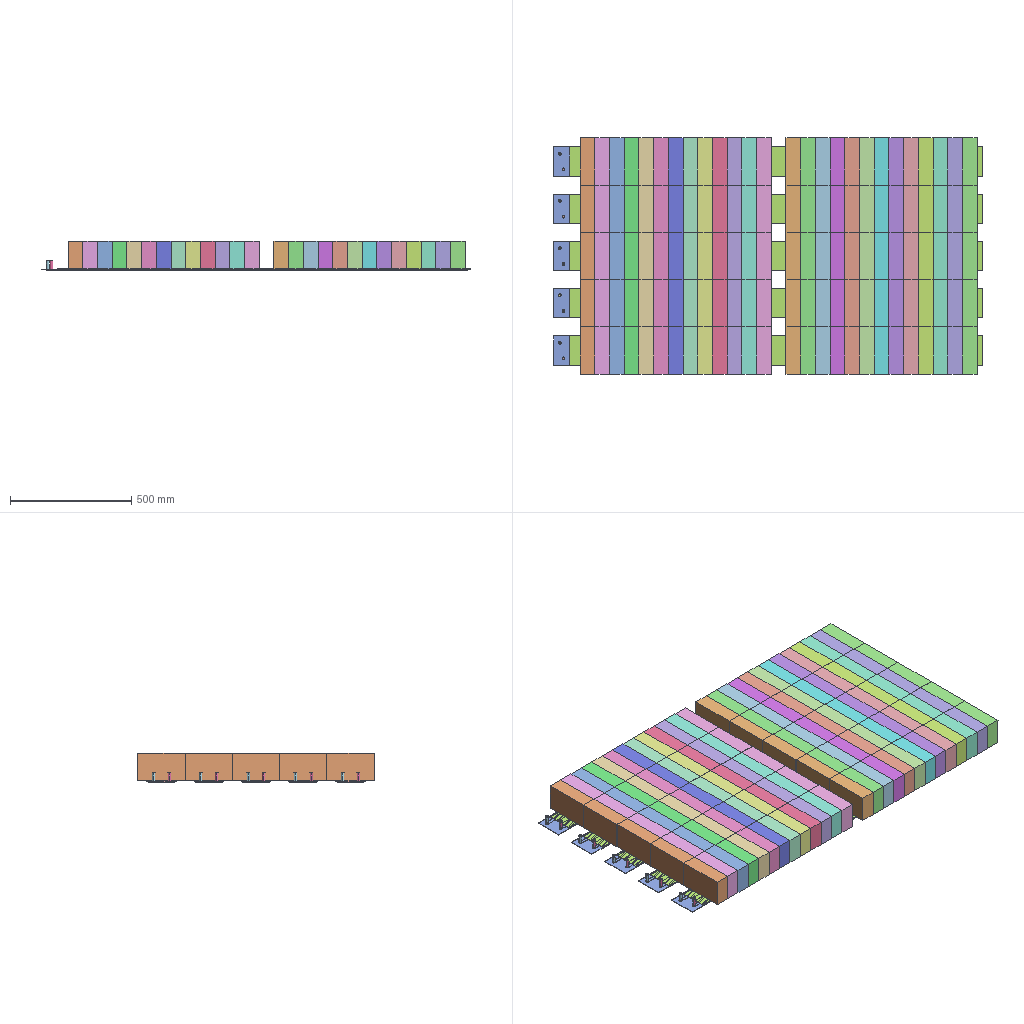Assembly | SolidWorks | 32 different items | 160 placed | box 1768 x 975 x 120 mm
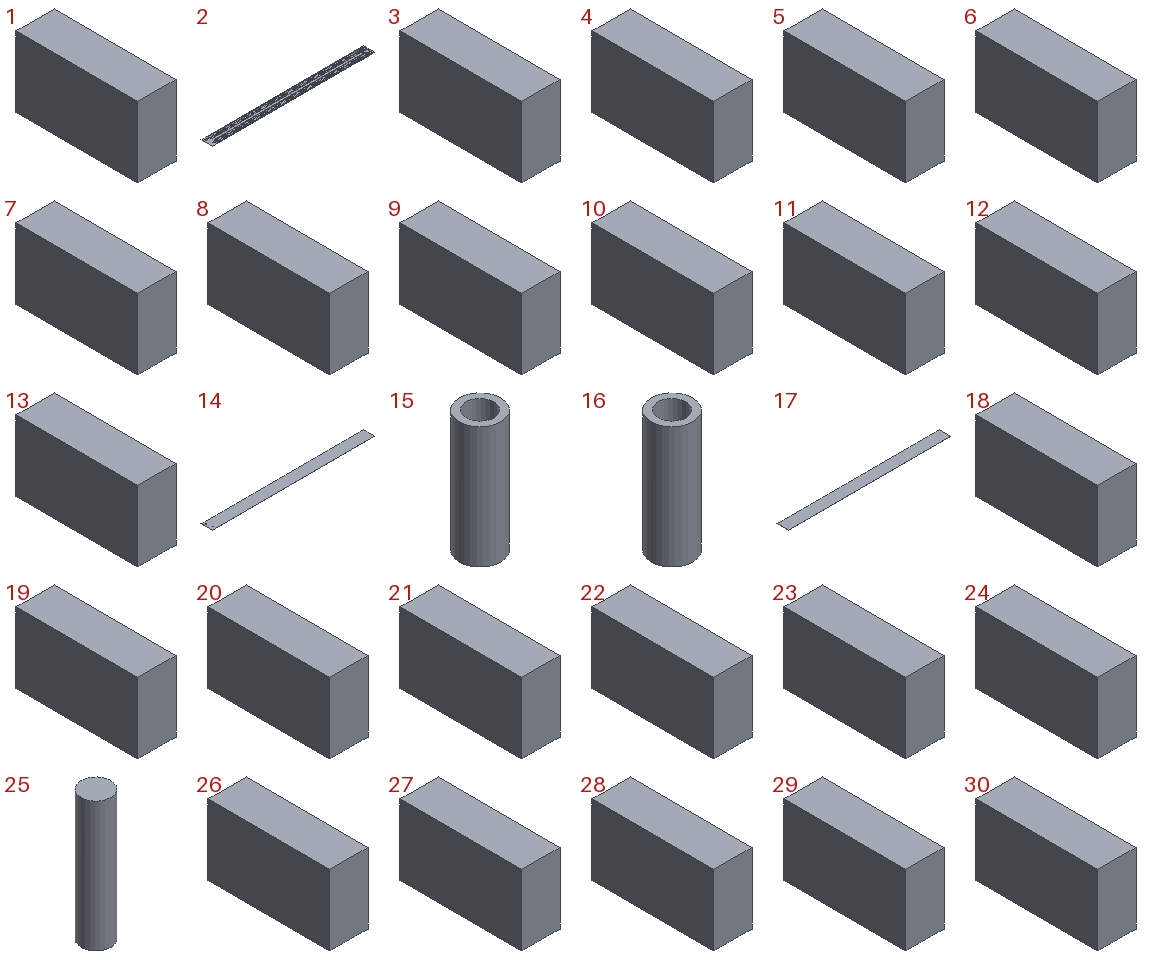Parts list (item | quantity | size | volume | features):
1 | x5 | 60.7 x 194.65 x 112.8 mm | 1332761 mm3 | features BaseBody 1
2 | x5 | 1768 x 120 x 5 mm | 284579 mm3 | features ICE 4, BaseBody 1, LPattern 1, MirrorPattern 1
3 | x5 | 60.7 x 194.65 x 112.8 mm | 1332761 mm3 | features BaseBody 1
4 | x5 | 60.7 x 194.65 x 112.8 mm | 1332761 mm3 | features BaseBody 1
5 | x5 | 60.7 x 194.65 x 112.8 mm | 1332761 mm3 | features BaseBody 1
6 | x5 | 60.7 x 194.65 x 112.8 mm | 1332761 mm3 | features BaseBody 1
7 | x5 | 60.7 x 194.65 x 112.8 mm | 1332761 mm3 | features BaseBody 1
8 | x5 | 60.7 x 194.65 x 112.8 mm | 1332761 mm3 | features BaseBody 1
9 | x5 | 60.7 x 194.65 x 112.8 mm | 1332761 mm3 | features BaseBody 1
10 | x5 | 60.7 x 194.65 x 112.8 mm | 1332761 mm3 | features BaseBody 1
11 | x5 | 60.7 x 194.65 x 112.8 mm | 1332761 mm3 | features BaseBody 1
12 | x5 | 60.7 x 194.65 x 112.8 mm | 1332761 mm3 | features BaseBody 1
13 | x5 | 60.7 x 194.65 x 112.8 mm | 1332761 mm3 | features BaseBody 1
14 | x5 | 1768 x 120 x 1 mm | 211934 mm3 | features BaseBody 1
15 | x5 | 12 x 12 x 35 mm | 2199 mm3 | features BaseBody 1
16 | x5 | 12 x 12 x 35 mm | 2199 mm3 | features BaseBody 1
17 | x5 | 1703 x 120 x 1 mm | 204360 mm3 | features BaseBody 1
18 | x5 | 60.7 x 194.65 x 112.8 mm | 1332761 mm3 | features BaseBody 1
19 | x5 | 60.7 x 194.65 x 112.8 mm | 1332761 mm3 | features BaseBody 1
20 | x5 | 60.7 x 194.65 x 112.8 mm | 1332761 mm3 | features BaseBody 1
21 | x5 | 60.7 x 194.65 x 112.8 mm | 1332761 mm3 | features BaseBody 1
22 | x5 | 60.7 x 194.65 x 112.8 mm | 1332761 mm3 | features BaseBody 1
23 | x5 | 60.7 x 194.65 x 112.8 mm | 1332761 mm3 | features BaseBody 1
24 | x5 | 60.7 x 194.65 x 112.8 mm | 1332761 mm3 | features BaseBody 1
25 | x5 | 8 x 8 x 35 mm | 1759 mm3 | features BaseBody 1
26 | x5 | 60.7 x 194.65 x 112.8 mm | 1332761 mm3 | features BaseBody 1
27 | x5 | 60.7 x 194.65 x 112.8 mm | 1332761 mm3 | features BaseBody 1
28 | x5 | 60.7 x 194.65 x 112.8 mm | 1332761 mm3 | features BaseBody 1
29 | x5 | 60.7 x 194.65 x 112.8 mm | 1332761 mm3 | features BaseBody 1
30 | x5 | 60.7 x 194.65 x 112.8 mm | 1332761 mm3 | features BaseBody 1
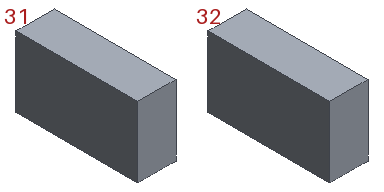31 | x5 | 60.7 x 194.65 x 112.8 mm | 1332761 mm3 | features BaseBody 1
32 | x5 | 60.7 x 194.65 x 112.8 mm | 1332761 mm3 | features BaseBody 1